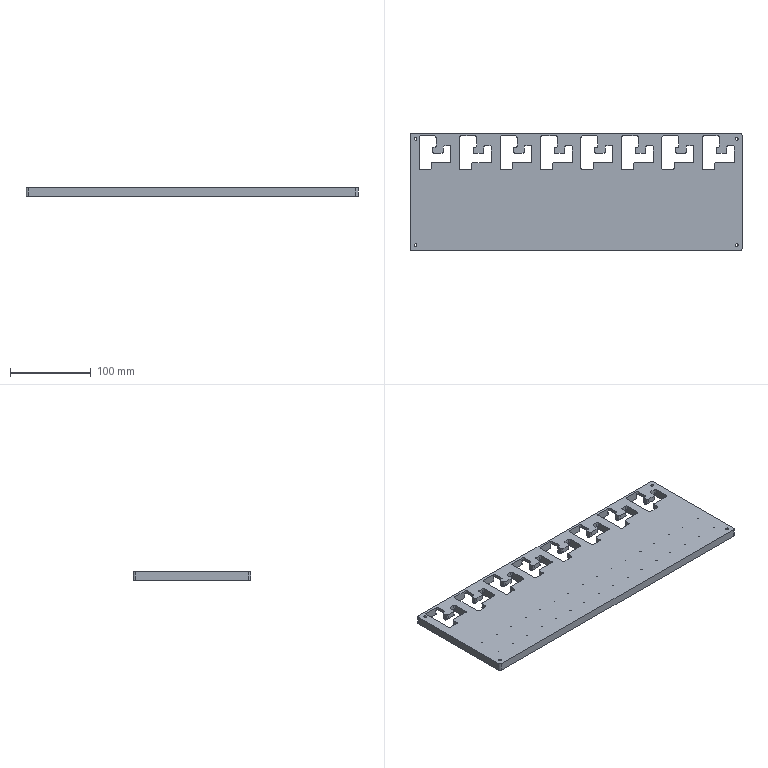NC program | NX | posted with a generic post | part box 410 x 145 x 10 mm
Lines 19770 to 19918 of 104733:
(DRILLING , TOOL : D6A45)
N39514 T07 M6
N39516 G54
N39518 G17 G0 G90 X-198. Y65.5 S5000 M3
N39520 G43 Z30. H7
N39522 G94 G81 G98 Z-1. F250. R3.
N39524 X-189.19 Y62.983
N39526 X-187.213 Y51.734 Z-3. R1.
N39528 X-183.226 Y46.729
N39530 X-187.213 Y23.734
N39532 X-161.213
N39534 X-165.407 Y27.955
N39536 X-161.213 Y51.734
N39538 X-159.194 Y62.88 Z-1. R3.
N39540 X-139.19 Y62.983
N39542 X-137.213 Y51.734 Z-3. R1.
N39544 X-133.226 Y46.729
N39546 X-137.213 Y23.734
N39548 X-111.213
N39550 X-115.407 Y27.955
N39552 X-111.213 Y51.734
N39554 X-109.194 Y62.88 Z-1. R3.
N39556 X-87.213 Y51.734 Z-3. R1.
N39558 X-83.226 Y46.729
N39560 X-87.213 Y23.734
N39562 X-65.407 Y27.955
N39564 X-61.213 Y23.734
N39566 X-37.213
N39568 X-33.226 Y46.729
N39570 X-37.213 Y51.734
N39572 X-61.213
N39574 X-59.194 Y62.88 Z-1. R3.
N39576 X-39.19 Y62.983
N39578 X-9.194 Y62.88
N39580 X-11.213 Y51.734 Z-3. R1.
N39582 X-15.407 Y27.955
N39584 X-11.213 Y23.734
N39586 X12.787
N39588 X38.787
N39590 X34.593 Y27.955
N39592 X16.774 Y46.729
N39594 X12.787 Y51.734
N39596 X10.81 Y62.983 Z-1. R3.
N39598 X38.787 Y51.734 Z-3. R1.
N39600 X40.806 Y62.88 Z-1. R3.
N39602 X60.81 Y62.983
N39604 X62.787 Y51.734 Z-3. R1.
N39606 X66.774 Y46.729
N39608 X62.787 Y23.734
N39610 X88.787
N39612 X84.593 Y27.955
N39614 X88.787 Y51.734
N39616 X90.806 Y62.88 Z-1. R3.
N39618 X110.81 Y62.983
N39620 X112.787 Y51.734 Z-3. R1.
N39622 X116.774 Y46.729
N39624 X112.787 Y23.734
N39626 X138.787
N39628 X134.593 Y27.955
N39630 X138.787 Y51.734
N39632 X140.806 Y62.88 Z-1. R3.
N39634 X160.81 Y62.983
N39636 X162.787 Y51.734 Z-3. R1.
N39638 X166.774 Y46.729
N39640 X190.806 Y62.88 Z-1. R3.
N39642 X198.5 Y65.5
N39644 X188.787 Y51.734 Z-3. R1.
N39646 X184.593 Y27.955
N39648 X188.787 Y23.734
N39650 X162.787
N39652 X198.5 Y-65.5 Z-1. R3.
N39654 X175.676 Y-53.441
N39656 X125.676
N39658 X75.676
N39660 X25.676
N39662 X-24.324
N39664 X-74.324
N39666 X-124.324
N39668 X-174.324
N39670 X-198. Y-65.5
N39672 G80
N39674 G0 X-198. Y-65.5 Z30.
N39676 M5
(DRILLING_COPY , TOOL : 3.2ZT)
N39678 T13 M6
N39680 G54
N39682 G17 G0 G90 X-198. Y65.5 S2000 M3
N39684 G43 Z30. H13
N39686 G94 G83 G98 Z-12.461 F150. Q2. R-0.5
N39688 Y-65.5
N39690 X198.5
N39692 Y65.5
N39694 G80
N39696 G0 X198.5 Y65.5 Z30.
N39698 M5
(DRILLING_COPY_COPY , TOOL : 1.59ZT)
N39700 T15 M6
N39702 G54
N39704 G17 G0 G90 X-187.213 Y51.734 S2000 M3
N39706 G43 Z30. H15
N39708 G94 G83 G98 Z-9.478 F150. Q2. R1.
N39710 X-161.213
N39712 X-137.213
N39714 X-111.213
N39716 X-87.213
N39718 X-61.213
N39720 X-37.213
N39722 X-11.213
N39724 X12.787
N39726 X38.787
N39728 X62.787
N39730 X88.787
N39732 X112.787
N39734 X138.787
N39736 X162.787
N39738 X188.787
N39740 Y23.734
N39742 X184.593 Y27.955 Z-8.
N39744 X162.787 Y23.734 Z-9.478
N39746 X138.787
N39748 X134.593 Y27.955 Z-8.
N39750 X112.787 Y23.734 Z-9.478
N39752 X88.787
N39754 X84.593 Y27.955 Z-8.
N39756 X62.787 Y23.734 Z-9.478
N39758 X38.787
N39760 X34.593 Y27.955 Z-8.
N39762 X12.787 Y23.734 Z-9.478
N39764 X-11.213
N39766 X-15.407 Y27.955 Z-8.
N39768 X-37.213 Y23.734 Z-9.478
N39770 X-61.213
N39772 X-65.407 Y27.955 Z-8.
N39774 X-87.213 Y23.734 Z-9.478
N39776 X-111.213
N39778 X-115.407 Y27.955 Z-8.
N39780 X-137.213 Y23.734 Z-9.478
N39782 X-161.213
N39784 X-165.407 Y27.955 Z-8.
N39786 X-187.213 Y23.734 Z-9.478
N39788 G80
N39790 G0 X-187.213 Y23.734 Z30.
N39792 M5